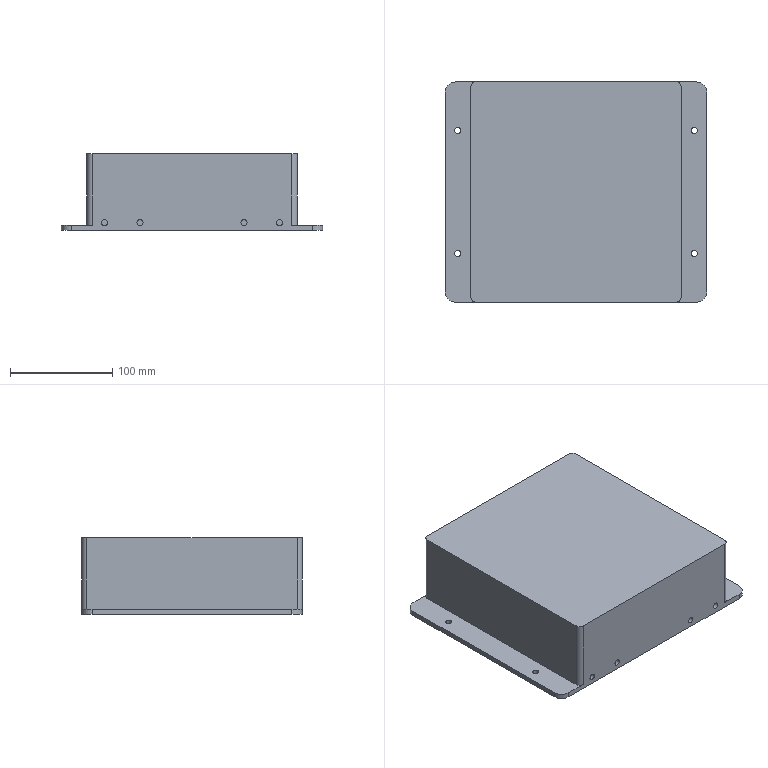NC program | NX | posted with a generic post | part box 255 x 215 x 75 mm
Lines 27 to 797 of 12583:
(ZLEVEL_PROFILE_COPY_1 , TOOL : D16)
N52 T18 M6
N54 G54
N56 G17 G0 G90 X-47.703 Y115.6 B0. C0. S8000 M3
N58 G43 Z30. H18
N60 Z1.5
N62 G94 G1 X0. Z-1. F1000.
N64 X117.5 F3000.
N66 G2 X135.6 Y97.5 R18.1
N68 G1 Y-97.5
N70 G2 X117.5 Y-115.6 R18.1
N72 G1 X-117.5
N74 G2 X-135.6 Y-97.5 R18.1
N76 G1 Y97.5
N78 G2 X-117.5 Y115.6 R18.1
N80 G1 X0.
N82 X117.5 Z-1.121
N84 X118.515 Y115.572 Z-1.122
N86 X119.527 Y115.486 Z-1.123
N88 X120.532 Y115.344 Z-1.124
N90 X121.528 Y115.146 Z-1.125
N92 X122.511 Y114.893 Z-1.126
N94 X123.478 Y114.584 Z-1.127
N96 X124.427 Y114.222 Z-1.128
N98 X125.353 Y113.808 Z-1.129
N100 X126.255 Y113.342 Z-1.13
N102 X127.13 Y112.826 Z-1.131
N104 X127.974 Y112.262 Z-1.132
N106 X128.785 Y111.651 Z-1.133
N108 X129.561 Y110.996 Z-1.134
N110 X130.299 Y110.299 Z-1.135
N112 X130.996 Y109.561 Z-1.136
N114 X131.651 Y108.785 Z-1.137
N116 X132.262 Y107.974 Z-1.138
N118 X132.826 Y107.13 Z-1.139
N120 X133.342 Y106.255 Z-1.14
N122 X133.808 Y105.353 Z-1.142
N124 X134.222 Y104.427 Z-1.143
N126 X134.584 Y103.478 Z-1.144
N128 X134.893 Y102.511 Z-1.145
N130 X135.146 Y101.528 Z-1.146
N132 X135.344 Y100.532 Z-1.147
N134 X135.486 Y99.527 Z-1.148
N136 X135.572 Y98.515 Z-1.149
N138 X135.6 Y97.5 Z-1.15
N140 Y-97.5 Z-1.35
N142 X135.572 Y-98.515 Z-1.351
N144 X135.486 Y-99.527 Z-1.352
N146 X135.344 Y-100.532 Z-1.353
N148 X135.146 Y-101.528 Z-1.354
N150 X134.893 Y-102.511 Z-1.355
N152 X134.584 Y-103.478 Z-1.356
N154 X134.222 Y-104.427 Z-1.357
N156 X133.808 Y-105.353 Z-1.358
N158 X133.342 Y-106.255 Z-1.36
N160 X132.826 Y-107.13 Z-1.361
N162 X132.262 Y-107.974 Z-1.362
N164 X131.651 Y-108.785 Z-1.363
N166 X130.996 Y-109.561 Z-1.364
N168 X130.299 Y-110.299 Z-1.365
N170 X129.561 Y-110.996 Z-1.366
N172 X128.785 Y-111.651 Z-1.367
N174 X127.974 Y-112.262 Z-1.368
N176 X127.13 Y-112.826 Z-1.369
N178 X126.255 Y-113.342 Z-1.37
N180 X125.353 Y-113.808 Z-1.371
N182 X124.427 Y-114.222 Z-1.372
N184 X123.478 Y-114.584 Z-1.373
N186 X122.511 Y-114.893 Z-1.374
N188 X121.528 Y-115.146 Z-1.375
N190 X120.532 Y-115.344 Z-1.376
N192 X119.527 Y-115.486 Z-1.377
N194 X118.515 Y-115.572 Z-1.378
N196 X117.5 Y-115.6 Z-1.379
N198 X-117.5 Z-1.621
N200 X-118.515 Y-115.572 Z-1.622
N202 X-119.527 Y-115.486 Z-1.623
N204 X-120.532 Y-115.344 Z-1.624
N206 X-121.528 Y-115.146 Z-1.625
N208 X-122.511 Y-114.893 Z-1.626
N210 X-123.478 Y-114.584 Z-1.627
N212 X-124.427 Y-114.222 Z-1.628
N214 X-125.353 Y-113.808 Z-1.629
N216 X-126.255 Y-113.342 Z-1.63
N218 X-127.13 Y-112.826 Z-1.631
N220 X-127.974 Y-112.262 Z-1.632
N222 X-128.785 Y-111.651 Z-1.633
N224 X-129.561 Y-110.996 Z-1.634
N226 X-130.299 Y-110.299 Z-1.635
N228 X-130.996 Y-109.561 Z-1.636
N230 X-131.651 Y-108.785 Z-1.637
N232 X-132.262 Y-107.974 Z-1.638
N234 X-132.826 Y-107.13 Z-1.639
N236 X-133.342 Y-106.255 Z-1.64
N238 X-133.808 Y-105.353 Z-1.642
N240 X-134.222 Y-104.427 Z-1.643
N242 X-134.584 Y-103.478 Z-1.644
N244 X-134.893 Y-102.511 Z-1.645
N246 X-135.146 Y-101.528 Z-1.646
N248 X-135.344 Y-100.532 Z-1.647
N250 X-135.486 Y-99.527 Z-1.648
N252 X-135.572 Y-98.515 Z-1.649
N254 X-135.6 Y-97.5 Z-1.65
N256 Y97.5 Z-1.85
N258 X-135.572 Y98.515 Z-1.851
N260 X-135.486 Y99.527 Z-1.852
N262 X-135.344 Y100.532 Z-1.853
N264 X-135.146 Y101.528 Z-1.854
N266 X-134.893 Y102.511 Z-1.855
N268 X-134.584 Y103.478 Z-1.856
N270 X-134.222 Y104.427 Z-1.857
N272 X-133.808 Y105.353 Z-1.858
N274 X-133.342 Y106.255 Z-1.86
N276 X-132.826 Y107.13 Z-1.861
N278 X-132.262 Y107.974 Z-1.862
N280 X-131.651 Y108.785 Z-1.863
N282 X-130.996 Y109.561 Z-1.864
N284 X-130.299 Y110.299 Z-1.865
N286 X-129.561 Y110.996 Z-1.866
N288 X-128.785 Y111.651 Z-1.867
N290 X-127.974 Y112.262 Z-1.868
N292 X-127.13 Y112.826 Z-1.869
N294 X-126.255 Y113.342 Z-1.87
N296 X-125.353 Y113.808 Z-1.871
N298 X-124.427 Y114.222 Z-1.872
N300 X-123.478 Y114.584 Z-1.873
N302 X-122.511 Y114.893 Z-1.874
N304 X-121.528 Y115.146 Z-1.875
N306 X-120.532 Y115.344 Z-1.876
N308 X-119.527 Y115.486 Z-1.877
N310 X-118.515 Y115.572 Z-1.878
N312 X-117.5 Y115.6 Z-1.879
N314 X0. Z-2.
N316 X117.5 Z-2.121
N318 X118.515 Y115.572 Z-2.122
N320 X119.527 Y115.486 Z-2.123
N322 X120.532 Y115.344 Z-2.124
N324 X121.528 Y115.146 Z-2.125
N326 X122.511 Y114.893 Z-2.126
N328 X123.478 Y114.584 Z-2.127
N330 X124.427 Y114.222 Z-2.128
N332 X125.353 Y113.808 Z-2.129
N334 X126.255 Y113.342 Z-2.13
N336 X127.13 Y112.826 Z-2.131
N338 X127.974 Y112.262 Z-2.132
N340 X128.785 Y111.651 Z-2.133
N342 X129.561 Y110.996 Z-2.134
N344 X130.299 Y110.299 Z-2.135
N346 X130.996 Y109.561 Z-2.136
N348 X131.651 Y108.785 Z-2.137
N350 X132.262 Y107.974 Z-2.138
N352 X132.826 Y107.13 Z-2.139
N354 X133.342 Y106.255 Z-2.14
N356 X133.808 Y105.353 Z-2.142
N358 X134.222 Y104.427 Z-2.143
N360 X134.584 Y103.478 Z-2.144
N362 X134.893 Y102.511 Z-2.145
N364 X135.146 Y101.528 Z-2.146
N366 X135.344 Y100.532 Z-2.147
N368 X135.486 Y99.527 Z-2.148
N370 X135.572 Y98.515 Z-2.149
N372 X135.6 Y97.5 Z-2.15
N374 Y-97.5 Z-2.35
N376 X135.572 Y-98.515 Z-2.351
N378 X135.486 Y-99.527 Z-2.352
N380 X135.344 Y-100.532 Z-2.353
N382 X135.146 Y-101.528 Z-2.354
N384 X134.893 Y-102.511 Z-2.355
N386 X134.584 Y-103.478 Z-2.356
N388 X134.222 Y-104.427 Z-2.357
N390 X133.808 Y-105.353 Z-2.358
N392 X133.342 Y-106.255 Z-2.36
N394 X132.826 Y-107.13 Z-2.361
N396 X132.262 Y-107.974 Z-2.362
N398 X131.651 Y-108.785 Z-2.363
N400 X130.996 Y-109.561 Z-2.364
N402 X130.299 Y-110.299 Z-2.365
N404 X129.561 Y-110.996 Z-2.366
N406 X128.785 Y-111.651 Z-2.367
N408 X127.974 Y-112.262 Z-2.368
N410 X127.13 Y-112.826 Z-2.369
N412 X126.255 Y-113.342 Z-2.37
N414 X125.353 Y-113.808 Z-2.371
N416 X124.427 Y-114.222 Z-2.372
N418 X123.478 Y-114.584 Z-2.373
N420 X122.511 Y-114.893 Z-2.374
N422 X121.528 Y-115.146 Z-2.375
N424 X120.532 Y-115.344 Z-2.376
N426 X119.527 Y-115.486 Z-2.377
N428 X118.515 Y-115.572 Z-2.378
N430 X117.5 Y-115.6 Z-2.379
N432 X-117.5 Z-2.621
N434 X-118.515 Y-115.572 Z-2.622
N436 X-119.527 Y-115.486 Z-2.623
N438 X-120.532 Y-115.344 Z-2.624
N440 X-121.528 Y-115.146 Z-2.625
N442 X-122.511 Y-114.893 Z-2.626
N444 X-123.478 Y-114.584 Z-2.627
N446 X-124.427 Y-114.222 Z-2.628
N448 X-125.353 Y-113.808 Z-2.629
N450 X-126.255 Y-113.342 Z-2.63
N452 X-127.13 Y-112.826 Z-2.631
N454 X-127.974 Y-112.262 Z-2.632
N456 X-128.785 Y-111.651 Z-2.633
N458 X-129.561 Y-110.996 Z-2.634
N460 X-130.299 Y-110.299 Z-2.635
N462 X-130.996 Y-109.561 Z-2.636
N464 X-131.651 Y-108.785 Z-2.637
N466 X-132.262 Y-107.974 Z-2.638
N468 X-132.826 Y-107.13 Z-2.639
N470 X-133.342 Y-106.255 Z-2.64
N472 X-133.808 Y-105.353 Z-2.642
N474 X-134.222 Y-104.427 Z-2.643
N476 X-134.584 Y-103.478 Z-2.644
N478 X-134.893 Y-102.511 Z-2.645
N480 X-135.146 Y-101.528 Z-2.646
N482 X-135.344 Y-100.532 Z-2.647
N484 X-135.486 Y-99.527 Z-2.648
N486 X-135.572 Y-98.515 Z-2.649
N488 X-135.6 Y-97.5 Z-2.65
N490 Y97.5 Z-2.85
N492 X-135.572 Y98.515 Z-2.851
N494 X-135.486 Y99.527 Z-2.852
N496 X-135.344 Y100.532 Z-2.853
N498 X-135.146 Y101.528 Z-2.854
N500 X-134.893 Y102.511 Z-2.855
N502 X-134.584 Y103.478 Z-2.856
N504 X-134.222 Y104.427 Z-2.857
N506 X-133.808 Y105.353 Z-2.858
N508 X-133.342 Y106.255 Z-2.86
N510 X-132.826 Y107.13 Z-2.861
N512 X-132.262 Y107.974 Z-2.862
N514 X-131.651 Y108.785 Z-2.863
N516 X-130.996 Y109.561 Z-2.864
N518 X-130.299 Y110.299 Z-2.865
N520 X-129.561 Y110.996 Z-2.866
N522 X-128.785 Y111.651 Z-2.867
N524 X-127.974 Y112.262 Z-2.868
N526 X-127.13 Y112.826 Z-2.869
N528 X-126.255 Y113.342 Z-2.87
N530 X-125.353 Y113.808 Z-2.871
N532 X-124.427 Y114.222 Z-2.872
N534 X-123.478 Y114.584 Z-2.873
N536 X-122.511 Y114.893 Z-2.874
N538 X-121.528 Y115.146 Z-2.875
N540 X-120.532 Y115.344 Z-2.876
N542 X-119.527 Y115.486 Z-2.877
N544 X-118.515 Y115.572 Z-2.878
N546 X-117.5 Y115.6 Z-2.879
N548 X0. Z-3.
N550 X117.5 Z-3.121
N552 X118.515 Y115.572 Z-3.122
N554 X119.527 Y115.486 Z-3.123
N556 X120.532 Y115.344 Z-3.124
N558 X121.528 Y115.146 Z-3.125
N560 X122.511 Y114.893 Z-3.126
N562 X123.478 Y114.584 Z-3.127
N564 X124.427 Y114.222 Z-3.128
N566 X125.353 Y113.808 Z-3.129
N568 X126.255 Y113.342 Z-3.13
N570 X127.13 Y112.826 Z-3.131
N572 X127.974 Y112.262 Z-3.132
N574 X128.785 Y111.651 Z-3.133
N576 X129.561 Y110.996 Z-3.134
N578 X130.299 Y110.299 Z-3.135
N580 X130.996 Y109.561 Z-3.136
N582 X131.651 Y108.785 Z-3.137
N584 X132.262 Y107.974 Z-3.138
N586 X132.826 Y107.13 Z-3.139
N588 X133.342 Y106.255 Z-3.14
N590 X133.808 Y105.353 Z-3.142
N592 X134.222 Y104.427 Z-3.143
N594 X134.584 Y103.478 Z-3.144
N596 X134.893 Y102.511 Z-3.145
N598 X135.146 Y101.528 Z-3.146
N600 X135.344 Y100.532 Z-3.147
N602 X135.486 Y99.527 Z-3.148
N604 X135.572 Y98.515 Z-3.149
N606 X135.6 Y97.5 Z-3.15
N608 Y-97.5 Z-3.35
N610 X135.572 Y-98.515 Z-3.351
N612 X135.486 Y-99.527 Z-3.352
N614 X135.344 Y-100.532 Z-3.353
N616 X135.146 Y-101.528 Z-3.354
N618 X134.893 Y-102.511 Z-3.355
N620 X134.584 Y-103.478 Z-3.356
N622 X134.222 Y-104.427 Z-3.357
N624 X133.808 Y-105.353 Z-3.358
N626 X133.342 Y-106.255 Z-3.36
N628 X132.826 Y-107.13 Z-3.361
N630 X132.262 Y-107.974 Z-3.362
N632 X131.651 Y-108.785 Z-3.363
N634 X130.996 Y-109.561 Z-3.364
N636 X130.299 Y-110.299 Z-3.365
N638 X129.561 Y-110.996 Z-3.366
N640 X128.785 Y-111.651 Z-3.367
N642 X127.974 Y-112.262 Z-3.368
N644 X127.13 Y-112.826 Z-3.369
N646 X126.255 Y-113.342 Z-3.37
N648 X125.353 Y-113.808 Z-3.371
N650 X124.427 Y-114.222 Z-3.372
N652 X123.478 Y-114.584 Z-3.373
N654 X122.511 Y-114.893 Z-3.374
N656 X121.528 Y-115.146 Z-3.375
N658 X120.532 Y-115.344 Z-3.376
N660 X119.527 Y-115.486 Z-3.377
N662 X118.515 Y-115.572 Z-3.378
N664 X117.5 Y-115.6 Z-3.379
N666 X-117.5 Z-3.621
N668 X-118.515 Y-115.572 Z-3.622
N670 X-119.527 Y-115.486 Z-3.623
N672 X-120.532 Y-115.344 Z-3.624
N674 X-121.528 Y-115.146 Z-3.625
N676 X-122.511 Y-114.893 Z-3.626
N678 X-123.478 Y-114.584 Z-3.627
N680 X-124.427 Y-114.222 Z-3.628
N682 X-125.353 Y-113.808 Z-3.629
N684 X-126.255 Y-113.342 Z-3.63
N686 X-127.13 Y-112.826 Z-3.631
N688 X-127.974 Y-112.262 Z-3.632
N690 X-128.785 Y-111.651 Z-3.633
N692 X-129.561 Y-110.996 Z-3.634
N694 X-130.299 Y-110.299 Z-3.635
N696 X-130.996 Y-109.561 Z-3.636
N698 X-131.651 Y-108.785 Z-3.637
N700 X-132.262 Y-107.974 Z-3.638
N702 X-132.826 Y-107.13 Z-3.639
N704 X-133.342 Y-106.255 Z-3.64
N706 X-133.808 Y-105.353 Z-3.642
N708 X-134.222 Y-104.427 Z-3.643
N710 X-134.584 Y-103.478 Z-3.644
N712 X-134.893 Y-102.511 Z-3.645
N714 X-135.146 Y-101.528 Z-3.646
N716 X-135.344 Y-100.532 Z-3.647
N718 X-135.486 Y-99.527 Z-3.648
N720 X-135.572 Y-98.515 Z-3.649
N722 X-135.6 Y-97.5 Z-3.65
N724 Y97.5 Z-3.85
N726 X-135.572 Y98.515 Z-3.851
N728 X-135.486 Y99.527 Z-3.852
N730 X-135.344 Y100.532 Z-3.853
N732 X-135.146 Y101.528 Z-3.854
N734 X-134.893 Y102.511 Z-3.855
N736 X-134.584 Y103.478 Z-3.856
N738 X-134.222 Y104.427 Z-3.857
N740 X-133.808 Y105.353 Z-3.858
N742 X-133.342 Y106.255 Z-3.86
N744 X-132.826 Y107.13 Z-3.861
N746 X-132.262 Y107.974 Z-3.862
N748 X-131.651 Y108.785 Z-3.863
N750 X-130.996 Y109.561 Z-3.864
N752 X-130.299 Y110.299 Z-3.865
N754 X-129.561 Y110.996 Z-3.866
N756 X-128.785 Y111.651 Z-3.867
N758 X-127.974 Y112.262 Z-3.868
N760 X-127.13 Y112.826 Z-3.869
N762 X-126.255 Y113.342 Z-3.87
N764 X-125.353 Y113.808 Z-3.871
N766 X-124.427 Y114.222 Z-3.872
N768 X-123.478 Y114.584 Z-3.873
N770 X-122.511 Y114.893 Z-3.874
N772 X-121.528 Y115.146 Z-3.875
N774 X-120.532 Y115.344 Z-3.876
N776 X-119.527 Y115.486 Z-3.877
N778 X-118.515 Y115.572 Z-3.878
N780 X-117.5 Y115.6 Z-3.879
N782 X0. Z-4.
N784 X117.5 Z-4.121
N786 X118.515 Y115.572 Z-4.122
N788 X119.527 Y115.486 Z-4.123
N790 X120.532 Y115.344 Z-4.124
N792 X121.528 Y115.146 Z-4.125
N794 X122.511 Y114.893 Z-4.126
N796 X123.478 Y114.584 Z-4.127
N798 X124.427 Y114.222 Z-4.128
N800 X125.353 Y113.808 Z-4.129
N802 X126.255 Y113.342 Z-4.13
N804 X127.13 Y112.826 Z-4.131
N806 X127.974 Y112.262 Z-4.132
N808 X128.785 Y111.651 Z-4.133
N810 X129.561 Y110.996 Z-4.134
N812 X130.299 Y110.299 Z-4.135
N814 X130.996 Y109.561 Z-4.136
N816 X131.651 Y108.785 Z-4.137
N818 X132.262 Y107.974 Z-4.138
N820 X132.826 Y107.13 Z-4.139
N822 X133.342 Y106.255 Z-4.14
N824 X133.808 Y105.353 Z-4.142
N826 X134.222 Y104.427 Z-4.143
N828 X134.584 Y103.478 Z-4.144
N830 X134.893 Y102.511 Z-4.145
N832 X135.146 Y101.528 Z-4.146
N834 X135.344 Y100.532 Z-4.147
N836 X135.486 Y99.527 Z-4.148
N838 X135.572 Y98.515 Z-4.149
N840 X135.6 Y97.5 Z-4.15
N842 Y-97.5 Z-4.35
N844 X135.572 Y-98.515 Z-4.351
N846 X135.486 Y-99.527 Z-4.352
N848 X135.344 Y-100.532 Z-4.353
N850 X135.146 Y-101.528 Z-4.354
N852 X134.893 Y-102.511 Z-4.355
N854 X134.584 Y-103.478 Z-4.356
N856 X134.222 Y-104.427 Z-4.357
N858 X133.808 Y-105.353 Z-4.358
N860 X133.342 Y-106.255 Z-4.36
N862 X132.826 Y-107.13 Z-4.361
N864 X132.262 Y-107.974 Z-4.362
N866 X131.651 Y-108.785 Z-4.363
N868 X130.996 Y-109.561 Z-4.364
N870 X130.299 Y-110.299 Z-4.365
N872 X129.561 Y-110.996 Z-4.366
N874 X128.785 Y-111.651 Z-4.367
N876 X127.974 Y-112.262 Z-4.368
N878 X127.13 Y-112.826 Z-4.369
N880 X126.255 Y-113.342 Z-4.37
N882 X125.353 Y-113.808 Z-4.371
N884 X124.427 Y-114.222 Z-4.372
N886 X123.478 Y-114.584 Z-4.373
N888 X122.511 Y-114.893 Z-4.374
N890 X121.528 Y-115.146 Z-4.375
N892 X120.532 Y-115.344 Z-4.376
N894 X119.527 Y-115.486 Z-4.377
N896 X118.515 Y-115.572 Z-4.378
N898 X117.5 Y-115.6 Z-4.379
N900 X-117.5 Z-4.621
N902 X-118.515 Y-115.572 Z-4.622
N904 X-119.527 Y-115.486 Z-4.623
N906 X-120.532 Y-115.344 Z-4.624
N908 X-121.528 Y-115.146 Z-4.625
N910 X-122.511 Y-114.893 Z-4.626
N912 X-123.478 Y-114.584 Z-4.627
N914 X-124.427 Y-114.222 Z-4.628
N916 X-125.353 Y-113.808 Z-4.629
N918 X-126.255 Y-113.342 Z-4.63
N920 X-127.13 Y-112.826 Z-4.631
N922 X-127.974 Y-112.262 Z-4.632
N924 X-128.785 Y-111.651 Z-4.633
N926 X-129.561 Y-110.996 Z-4.634
N928 X-130.299 Y-110.299 Z-4.635
N930 X-130.996 Y-109.561 Z-4.636
N932 X-131.651 Y-108.785 Z-4.637
N934 X-132.262 Y-107.974 Z-4.638
N936 X-132.826 Y-107.13 Z-4.639
N938 X-133.342 Y-106.255 Z-4.64
N940 X-133.808 Y-105.353 Z-4.642
N942 X-134.222 Y-104.427 Z-4.643
N944 X-134.584 Y-103.478 Z-4.644
N946 X-134.893 Y-102.511 Z-4.645
N948 X-135.146 Y-101.528 Z-4.646
N950 X-135.344 Y-100.532 Z-4.647
N952 X-135.486 Y-99.527 Z-4.648
N954 X-135.572 Y-98.515 Z-4.649
N956 X-135.6 Y-97.5 Z-4.65
N958 Y97.5 Z-4.85
N960 X-135.572 Y98.515 Z-4.851
N962 X-135.486 Y99.527 Z-4.852
N964 X-135.344 Y100.532 Z-4.853
N966 X-135.146 Y101.528 Z-4.854
N968 X-134.893 Y102.511 Z-4.855
N970 X-134.584 Y103.478 Z-4.856
N972 X-134.222 Y104.427 Z-4.857
N974 X-133.808 Y105.353 Z-4.858
N976 X-133.342 Y106.255 Z-4.86
N978 X-132.826 Y107.13 Z-4.861
N980 X-132.262 Y107.974 Z-4.862
N982 X-131.651 Y108.785 Z-4.863
N984 X-130.996 Y109.561 Z-4.864
N986 X-130.299 Y110.299 Z-4.865
N988 X-129.561 Y110.996 Z-4.866
N990 X-128.785 Y111.651 Z-4.867
N992 X-127.974 Y112.262 Z-4.868
N994 X-127.13 Y112.826 Z-4.869
N996 X-126.255 Y113.342 Z-4.87
N998 X-125.353 Y113.808 Z-4.871
N1000 X-124.427 Y114.222 Z-4.872
N1002 X-123.478 Y114.584 Z-4.873
N1004 X-122.511 Y114.893 Z-4.874
N1006 X-121.528 Y115.146 Z-4.875
N1008 X-120.532 Y115.344 Z-4.876
N1010 X-119.527 Y115.486 Z-4.877
N1012 X-118.515 Y115.572 Z-4.878
N1014 X-117.5 Y115.6 Z-4.879
N1016 X0. Z-5.
N1018 X117.5 Z-5.121
N1020 X118.515 Y115.572 Z-5.122
N1022 X119.527 Y115.486 Z-5.123
N1024 X120.532 Y115.344 Z-5.124
N1026 X121.528 Y115.146 Z-5.125
N1028 X122.511 Y114.893 Z-5.126
N1030 X123.478 Y114.584 Z-5.127
N1032 X124.427 Y114.222 Z-5.128
N1034 X125.353 Y113.808 Z-5.129
N1036 X126.255 Y113.342 Z-5.13
N1038 X127.13 Y112.826 Z-5.131
N1040 X127.974 Y112.262 Z-5.132
N1042 X128.785 Y111.651 Z-5.133
N1044 X129.561 Y110.996 Z-5.134
N1046 X130.299 Y110.299 Z-5.135
N1048 X130.996 Y109.561 Z-5.136
N1050 X131.651 Y108.785 Z-5.137
N1052 X132.262 Y107.974 Z-5.138
N1054 X132.826 Y107.13 Z-5.139
N1056 X133.342 Y106.255 Z-5.14
N1058 X133.808 Y105.353 Z-5.142
N1060 X134.222 Y104.427 Z-5.143
N1062 X134.584 Y103.478 Z-5.144
N1064 X134.893 Y102.511 Z-5.145
N1066 X135.146 Y101.528 Z-5.146
N1068 X135.344 Y100.532 Z-5.147
N1070 X135.486 Y99.527 Z-5.148
N1072 X135.572 Y98.515 Z-5.149
N1074 X135.6 Y97.5 Z-5.15
N1076 Y-97.5 Z-5.35
N1078 X135.572 Y-98.515 Z-5.351
N1080 X135.486 Y-99.527 Z-5.352
N1082 X135.344 Y-100.532 Z-5.353
N1084 X135.146 Y-101.528 Z-5.354
N1086 X134.893 Y-102.511 Z-5.355
N1088 X134.584 Y-103.478 Z-5.356
N1090 X134.222 Y-104.427 Z-5.357
N1092 X133.808 Y-105.353 Z-5.358
N1094 X133.342 Y-106.255 Z-5.36
N1096 X132.826 Y-107.13 Z-5.361
N1098 X132.262 Y-107.974 Z-5.362
N1100 X131.651 Y-108.785 Z-5.363
N1102 X130.996 Y-109.561 Z-5.364
N1104 X130.299 Y-110.299 Z-5.365
N1106 X129.561 Y-110.996 Z-5.366
N1108 X128.785 Y-111.651 Z-5.367
N1110 X127.974 Y-112.262 Z-5.368
N1112 X127.13 Y-112.826 Z-5.369
N1114 X126.255 Y-113.342 Z-5.37
N1116 X125.353 Y-113.808 Z-5.371
N1118 X124.427 Y-114.222 Z-5.372
N1120 X123.478 Y-114.584 Z-5.373
N1122 X122.511 Y-114.893 Z-5.374
N1124 X121.528 Y-115.146 Z-5.375
N1126 X120.532 Y-115.344 Z-5.376
N1128 X119.527 Y-115.486 Z-5.377
N1130 X118.515 Y-115.572 Z-5.378
N1132 X117.5 Y-115.6 Z-5.379
N1134 X-117.5 Z-5.621
N1136 X-118.515 Y-115.572 Z-5.622
N1138 X-119.527 Y-115.486 Z-5.623
N1140 X-120.532 Y-115.344 Z-5.624
N1142 X-121.528 Y-115.146 Z-5.625
N1144 X-122.511 Y-114.893 Z-5.626
N1146 X-123.478 Y-114.584 Z-5.627
N1148 X-124.427 Y-114.222 Z-5.628
N1150 X-125.353 Y-113.808 Z-5.629
N1152 X-126.255 Y-113.342 Z-5.63
N1154 X-127.13 Y-112.826 Z-5.631
N1156 X-127.974 Y-112.262 Z-5.632
N1158 X-128.785 Y-111.651 Z-5.633
N1160 X-129.561 Y-110.996 Z-5.634
N1162 X-130.299 Y-110.299 Z-5.635
N1164 X-130.996 Y-109.561 Z-5.636
N1166 X-131.651 Y-108.785 Z-5.637
N1168 X-132.262 Y-107.974 Z-5.638
N1170 X-132.826 Y-107.13 Z-5.639
N1172 X-133.342 Y-106.255 Z-5.64
N1174 X-133.808 Y-105.353 Z-5.642
N1176 X-134.222 Y-104.427 Z-5.643
N1178 X-134.584 Y-103.478 Z-5.644
N1180 X-134.893 Y-102.511 Z-5.645
N1182 X-135.146 Y-101.528 Z-5.646
N1184 X-135.344 Y-100.532 Z-5.647
N1186 X-135.486 Y-99.527 Z-5.648
N1188 X-135.572 Y-98.515 Z-5.649
N1190 X-135.6 Y-97.5 Z-5.65
N1192 Y97.5 Z-5.85
N1194 X-135.572 Y98.515 Z-5.851
N1196 X-135.486 Y99.527 Z-5.852
N1198 X-135.344 Y100.532 Z-5.853
N1200 X-135.146 Y101.528 Z-5.854
N1202 X-134.893 Y102.511 Z-5.855
N1204 X-134.584 Y103.478 Z-5.856
N1206 X-134.222 Y104.427 Z-5.857
N1208 X-133.808 Y105.353 Z-5.858
N1210 X-133.342 Y106.255 Z-5.86
N1212 X-132.826 Y107.13 Z-5.861
N1214 X-132.262 Y107.974 Z-5.862
N1216 X-131.651 Y108.785 Z-5.863
N1218 X-130.996 Y109.561 Z-5.864
N1220 X-130.299 Y110.299 Z-5.865
N1222 X-129.561 Y110.996 Z-5.866
N1224 X-128.785 Y111.651 Z-5.867
N1226 X-127.974 Y112.262 Z-5.868
N1228 X-127.13 Y112.826 Z-5.869
N1230 X-126.255 Y113.342 Z-5.87
N1232 X-125.353 Y113.808 Z-5.871
N1234 X-124.427 Y114.222 Z-5.872
N1236 X-123.478 Y114.584 Z-5.873
N1238 X-122.511 Y114.893 Z-5.874
N1240 X-121.528 Y115.146 Z-5.875
N1242 X-120.532 Y115.344 Z-5.876
N1244 X-119.527 Y115.486 Z-5.877
N1246 X-118.515 Y115.572 Z-5.878
N1248 X-117.5 Y115.6 Z-5.879
N1250 X0. Z-6.
N1252 X117.5 Z-6.121
N1254 X118.515 Y115.572 Z-6.122
N1256 X119.527 Y115.486 Z-6.123
N1258 X120.532 Y115.344 Z-6.124
N1260 X121.528 Y115.146 Z-6.125
N1262 X122.511 Y114.893 Z-6.126
N1264 X123.478 Y114.584 Z-6.127
N1266 X124.427 Y114.222 Z-6.128
N1268 X125.353 Y113.808 Z-6.129
N1270 X126.255 Y113.342 Z-6.13
N1272 X127.13 Y112.826 Z-6.131
N1274 X127.974 Y112.262 Z-6.132
N1276 X128.785 Y111.651 Z-6.133
N1278 X129.561 Y110.996 Z-6.134
N1280 X130.299 Y110.299 Z-6.135
N1282 X130.996 Y109.561 Z-6.136
N1284 X131.651 Y108.785 Z-6.137
N1286 X132.262 Y107.974 Z-6.138
N1288 X132.826 Y107.13 Z-6.139
N1290 X133.342 Y106.255 Z-6.14
N1292 X133.808 Y105.353 Z-6.142
N1294 X134.222 Y104.427 Z-6.143
N1296 X134.584 Y103.478 Z-6.144
N1298 X134.893 Y102.511 Z-6.145
N1300 X135.146 Y101.528 Z-6.146
N1302 X135.344 Y100.532 Z-6.147
N1304 X135.486 Y99.527 Z-6.148
N1306 X135.572 Y98.515 Z-6.149
N1308 X135.6 Y97.5 Z-6.15
N1310 Y-97.5 Z-6.35
N1312 X135.572 Y-98.515 Z-6.351
N1314 X135.486 Y-99.527 Z-6.352
N1316 X135.344 Y-100.532 Z-6.353
N1318 X135.146 Y-101.528 Z-6.354
N1320 X134.893 Y-102.511 Z-6.355
N1322 X134.584 Y-103.478 Z-6.356
N1324 X134.222 Y-104.427 Z-6.357
N1326 X133.808 Y-105.353 Z-6.358
N1328 X133.342 Y-106.255 Z-6.36
N1330 X132.826 Y-107.13 Z-6.361
N1332 X132.262 Y-107.974 Z-6.362
N1334 X131.651 Y-108.785 Z-6.363
N1336 X130.996 Y-109.561 Z-6.364
N1338 X130.299 Y-110.299 Z-6.365
N1340 X129.561 Y-110.996 Z-6.366
N1342 X128.785 Y-111.651 Z-6.367
N1344 X127.974 Y-112.262 Z-6.368
N1346 X127.13 Y-112.826 Z-6.369
N1348 X126.255 Y-113.342 Z-6.37
N1350 X125.353 Y-113.808 Z-6.371
N1352 X124.427 Y-114.222 Z-6.372
N1354 X123.478 Y-114.584 Z-6.373
N1356 X122.511 Y-114.893 Z-6.374
N1358 X121.528 Y-115.146 Z-6.375
N1360 X120.532 Y-115.344 Z-6.376
N1362 X119.527 Y-115.486 Z-6.377
N1364 X118.515 Y-115.572 Z-6.378
N1366 X117.5 Y-115.6 Z-6.379
N1368 X-117.5 Z-6.621
N1370 X-118.515 Y-115.572 Z-6.622
N1372 X-119.527 Y-115.486 Z-6.623
N1374 X-120.532 Y-115.344 Z-6.624
N1376 X-121.528 Y-115.146 Z-6.625
N1378 X-122.511 Y-114.893 Z-6.626
N1380 X-123.478 Y-114.584 Z-6.627
N1382 X-124.427 Y-114.222 Z-6.628
N1384 X-125.353 Y-113.808 Z-6.629
N1386 X-126.255 Y-113.342 Z-6.63
N1388 X-127.13 Y-112.826 Z-6.631
N1390 X-127.974 Y-112.262 Z-6.632
N1392 X-128.785 Y-111.651 Z-6.633
N1394 X-129.561 Y-110.996 Z-6.634
N1396 X-130.299 Y-110.299 Z-6.635
N1398 X-130.996 Y-109.561 Z-6.636
N1400 X-131.651 Y-108.785 Z-6.637
N1402 X-132.262 Y-107.974 Z-6.638
N1404 X-132.826 Y-107.13 Z-6.639
N1406 X-133.342 Y-106.255 Z-6.64
N1408 X-133.808 Y-105.353 Z-6.642
N1410 X-134.222 Y-104.427 Z-6.643
N1412 X-134.584 Y-103.478 Z-6.644
N1414 X-134.893 Y-102.511 Z-6.645
N1416 X-135.146 Y-101.528 Z-6.646
N1418 X-135.344 Y-100.532 Z-6.647
N1420 X-135.486 Y-99.527 Z-6.648
N1422 X-135.572 Y-98.515 Z-6.649
N1424 X-135.6 Y-97.5 Z-6.65
N1426 Y97.5 Z-6.85
N1428 X-135.572 Y98.515 Z-6.851
N1430 X-135.486 Y99.527 Z-6.852
N1432 X-135.344 Y100.532 Z-6.853
N1434 X-135.146 Y101.528 Z-6.854
N1436 X-134.893 Y102.511 Z-6.855
N1438 X-134.584 Y103.478 Z-6.856
N1440 X-134.222 Y104.427 Z-6.857
N1442 X-133.808 Y105.353 Z-6.858
N1444 X-133.342 Y106.255 Z-6.86
N1446 X-132.826 Y107.13 Z-6.861
N1448 X-132.262 Y107.974 Z-6.862
N1450 X-131.651 Y108.785 Z-6.863
N1452 X-130.996 Y109.561 Z-6.864
N1454 X-130.299 Y110.299 Z-6.865
N1456 X-129.561 Y110.996 Z-6.866
N1458 X-128.785 Y111.651 Z-6.867
N1460 X-127.974 Y112.262 Z-6.868
N1462 X-127.13 Y112.826 Z-6.869
N1464 X-126.255 Y113.342 Z-6.87
N1466 X-125.353 Y113.808 Z-6.871
N1468 X-124.427 Y114.222 Z-6.872
N1470 X-123.478 Y114.584 Z-6.873
N1472 X-122.511 Y114.893 Z-6.874
N1474 X-121.528 Y115.146 Z-6.875
N1476 X-120.532 Y115.344 Z-6.876
N1478 X-119.527 Y115.486 Z-6.877
N1480 X-118.515 Y115.572 Z-6.878
N1482 X-117.5 Y115.6 Z-6.879
N1484 X0. Z-7.
N1486 X117.5 Z-7.121
N1488 X118.515 Y115.572 Z-7.122
N1490 X119.527 Y115.486 Z-7.123
N1492 X120.532 Y115.344 Z-7.124
N1494 X121.528 Y115.146 Z-7.125
N1496 X122.511 Y114.893 Z-7.126
N1498 X123.478 Y114.584 Z-7.127
N1500 X124.427 Y114.222 Z-7.128
N1502 X125.353 Y113.808 Z-7.129
N1504 X126.255 Y113.342 Z-7.13
N1506 X127.13 Y112.826 Z-7.131
N1508 X127.974 Y112.262 Z-7.132
N1510 X128.785 Y111.651 Z-7.133
N1512 X129.561 Y110.996 Z-7.134
N1514 X130.299 Y110.299 Z-7.135
N1516 X130.996 Y109.561 Z-7.136
N1518 X131.651 Y108.785 Z-7.137
N1520 X132.262 Y107.974 Z-7.138
N1522 X132.826 Y107.13 Z-7.139
N1524 X133.342 Y106.255 Z-7.14
N1526 X133.808 Y105.353 Z-7.142
N1528 X134.222 Y104.427 Z-7.143
N1530 X134.584 Y103.478 Z-7.144
N1532 X134.893 Y102.511 Z-7.145
N1534 X135.146 Y101.528 Z-7.146
N1536 X135.344 Y100.532 Z-7.147
N1538 X135.486 Y99.527 Z-7.148
N1540 X135.572 Y98.515 Z-7.149
N1542 X135.6 Y97.5 Z-7.15
N1544 Y-97.5 Z-7.35
N1546 X135.572 Y-98.515 Z-7.351
N1548 X135.486 Y-99.527 Z-7.352
N1550 X135.344 Y-100.532 Z-7.353
N1552 X135.146 Y-101.528 Z-7.354
N1554 X134.893 Y-102.511 Z-7.355
N1556 X134.584 Y-103.478 Z-7.356
N1558 X134.222 Y-104.427 Z-7.357
N1560 X133.808 Y-105.353 Z-7.358
N1562 X133.342 Y-106.255 Z-7.36
N1564 X132.826 Y-107.13 Z-7.361
N1566 X132.262 Y-107.974 Z-7.362
N1568 X131.651 Y-108.785 Z-7.363
N1570 X130.996 Y-109.561 Z-7.364
N1572 X130.299 Y-110.299 Z-7.365
N1574 X129.561 Y-110.996 Z-7.366
N1576 X128.785 Y-111.651 Z-7.367
N1578 X127.974 Y-112.262 Z-7.368
N1580 X127.13 Y-112.826 Z-7.369
N1582 X126.255 Y-113.342 Z-7.37
N1584 X125.353 Y-113.808 Z-7.371
N1586 X124.427 Y-114.222 Z-7.372